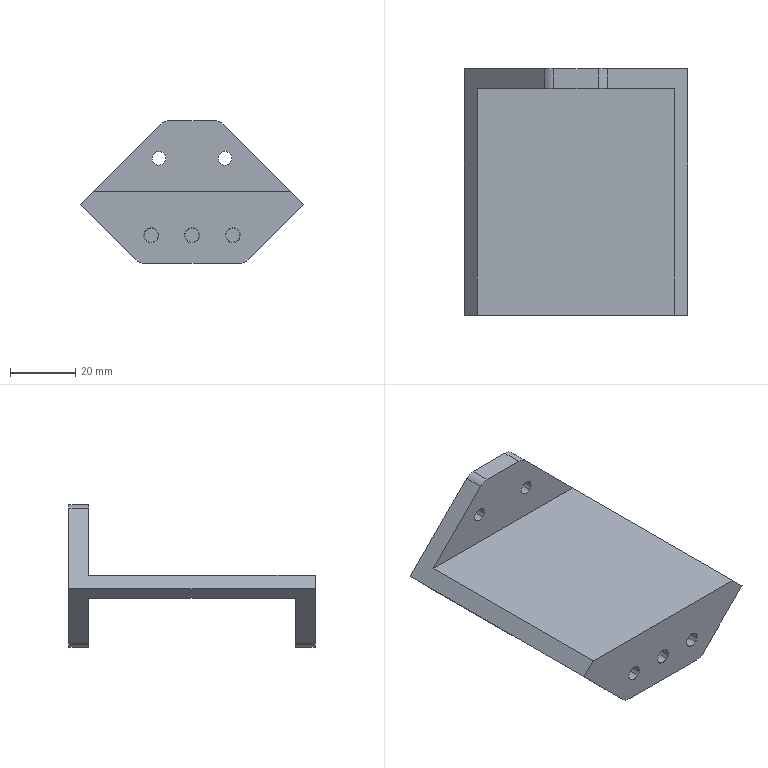NC program | NX | posted with a generic post | part box 68.307 x 75.3 x 43.668 mm
Lines 81 to 1013 of 6865:
(ADAPTIVE_MILLING_COPY_1 , TOOL : D10)
N160 T15 M6
N162 G54
N164 G17 G0 G90 X37.103 Y44.955 B0. C0. S9500 M3
N166 G43 Z30. H15
N168 Z-18.118
N170 G94 G1 Z-21.118 F1000.
N172 X35.037 Y43.518 F3000.
N174 G3 X34.603 Y42.688 R1.025
N176 G2 X37.336 Y37.585 R9.953
N178 X38.066 Y30.26 R36.076
N180 X38.139 Y16.26 R733.485
N182 G1 X38.14 Y-34.615
N184 X38.139 Y-34.74
N186 X38.135 Y-34.865
N188 X38.126 Y-34.99
N190 G2 X35.464 Y-39.18 R5.882
N192 X29.738 Y-41.187 R13.119
N194 X21.129 Y-41.612 R70.953
N196 G1 X19.879 Y-41.62
N198 X18.254 Y-41.627
N200 X16.004 Y-41.632
N202 X12.254 Y-41.636
N204 X0.629 Y-41.637
N206 X-31.121
N208 G2 X-35.385 Y-39.36 R5.577
N210 X-37.569 Y-33.972 R11.776
N212 X-38.106 Y-25.498 R55.2
N214 G1 X-38.116 Y-24.373
N216 X-38.125 Y-22.998
N218 X-38.132 Y-21.373
N220 X-38.136 Y-18.998
N222 X-38.139 Y-14.748
N224 X-38.14 Y7.252
N226 Y34.627
N228 X-38.135 Y34.877
N230 X-38.129 Y35.002
N232 X-38.118 Y35.126
N234 G2 X-36.378 Y38.941 R7.536
N236 G3 X-34.707 Y41.121 R26.03
N238 G1 X-34.661 Y41.238
N240 X-34.628 Y41.358
N242 X-34.606 Y41.481
N244 G3 X-35.484 Y42.483 R1.015
N246 G1 X-37.241 Y42.713
N248 G2 X-37.126 Y44.725 R1.01
N250 G1 Z-18.118
N252 G0 Z30.
N254 X37.103 Y45.944
N256 Z-18.118
N258 G1 Z-21.118 F1000.
N260 G2 X37.257 Y43.934 R1.01 F3000.
N262 G1 X35.476 Y43.689
N264 G3 X34.603 Y42.688 R1.015
N266 G2 X36.175 Y37.422 R55.918
N268 X37.056 Y27.727 R51.989
N270 X37.129 Y12.227 R790.085
N272 G1 Y-31.523
N274 X37.128 Y-31.648
N276 X37.126 Y-31.773
N278 X37.122 Y-31.898
N280 X37.116 Y-32.023
N282 X37.108 Y-32.147
N284 G2 X33.457 Y-37.968 R7.678
N286 X27.114 Y-40.112 R15.441
N288 X18.258 Y-40.59 R72.293
N290 G1 X17.133 Y-40.601
N292 X15.758 Y-40.61
N294 X14.008 Y-40.617
N296 X11.508 Y-40.622
N298 X7.508 Y-40.625
N300 X-4.742 Y-40.626
N302 X-27.992
N304 X-28.242 Y-40.624
N306 X-28.492 Y-40.615
N308 X-28.617 Y-40.606
N310 G2 X-34.521 Y-36.878 R7.68
N312 X-36.629 Y-30.521 R15.721
N314 X-37.101 Y-20.914 R80.427
N316 G1 X-37.11 Y-19.664
N318 X-37.117 Y-18.164
N320 X-37.123 Y-16.039
N322 X-37.127 Y-12.914
N324 X-37.129 Y-6.289
N326 Y31.711
N328 G2 X-35.536 Y37.429 R11.91
N330 G3 X-34.613 Y39.337 R10.413
N332 G1 X-34.603 Y39.41
N334 Y42.785
N336 G3 X-35.422 Y43.776 R1.017
N338 G1 X-36.981 Y44.078
N340 G3 X-37.127 Y42.077 R-1.01
N342 G1 Z-18.118
N344 G0 Z30.
N346 X37.103 Y45.449
N348 Z-18.118
N350 G1 Z-21.118 F1000.
N352 G2 X36.95 Y43.45 R-1.01 F3000.
N354 G1 X36.302 Y43.585
N356 X35.651 Y43.698
N358 G3 X34.603 Y42.688 R1.014
N360 X35.031 Y38.469 R20.052
N362 G2 X36.066 Y24.898 R85.494
N364 G1 X36.079 Y23.773
N366 X36.09 Y22.523
N368 X36.099 Y21.023
N370 X36.107 Y19.148
N372 X36.112 Y16.773
N374 X36.116 Y13.148
N376 X36.118 Y5.523
N378 X36.119 Y-28.852
N380 X36.117 Y-29.102
N382 X36.116 Y-29.227
N384 X36.113 Y-29.352
N386 X36.104 Y-29.602
N388 G2 X31.382 Y-37.073 R8.907
N390 X24.358 Y-39.151 R18.458
N392 X14.498 Y-39.586 R94.216
N394 G1 X13.123 Y-39.596
N396 X11.373 Y-39.604
N398 X9.123 Y-39.609
N400 X5.748 Y-39.613
N402 X-1.502 Y-39.615
N404 X-25.377
N406 G2 X-33.587 Y-34.86 R8.944
N408 X-35.64 Y-27.957 R18.351
N410 X-36.097 Y-16.972 R100.614
N412 G1 X-36.105 Y-15.347
N414 X-36.111 Y-13.222
N416 X-36.115 Y-10.222
N418 X-36.118 Y-4.597
N420 X-36.119 Y29.278
N422 X-36.116 Y29.528
N424 G2 X-34.835 Y35.861 R17.736
N426 X-34.752 Y38.412 R38.327
N428 G3 X-34.603 Y39.452 R4.992
N430 X-35.485 Y40.454 R1.015
N432 G1 X-37.225 Y40.677
N434 G2 X-37.127 Y42.689 R1.01
N436 G1 Z-18.118
N438 G0 Z30.
N440 X37.103 Y44.944
N442 Z-18.118
N444 G1 Z-21.118 F1000.
N446 G2 X37.27 Y42.934 R1.01 F3000.
N448 G1 X35.477 Y42.689
N450 G3 X34.603 Y41.688 R1.015
N452 G1 Y39.202
N454 X34.628 Y38.974
N456 G2 X34.815 Y37.63 R7.436
N458 G3 X35.002 Y27.258 R244.674
N460 G2 X35.107 Y4.883 R986.977
N462 G1 X35.108 Y-26.492
N464 X35.106 Y-26.867
N466 X35.102 Y-27.117
N468 X35.099 Y-27.242
N470 X35.09 Y-27.492
N472 X35.085 Y-27.616
N474 G2 X29.711 Y-36.054 R9.801
N476 X22.669 Y-38.093 R19.794
N478 X12.185 Y-38.573 R97.324
N480 G1 X10.81 Y-38.583
N482 X9.06 Y-38.591
N484 X6.685 Y-38.598
N486 X3.435 Y-38.602
N488 X-2.815 Y-38.604
N490 X-23.065 Y-38.605
N492 G2 X-29.137 Y-37.029 R10.422
N494 X-33.535 Y-30.968 R11.649
N496 X-34.886 Y-22.856 R30.289
N498 X-35.105 Y-7.234 R329.937
N500 G1 X-35.107 Y-1.359
N502 X-35.108 Y27.141
N504 X-35.107 Y27.391
N506 X-35.098 Y27.891
N508 X-35.089 Y28.266
N510 G2 X-34.789 Y31.456 R37.745
N512 G1 X-34.815 Y36.061
N514 G3 X-35.651 Y37.056 R1.016
N516 G1 X-37.096 Y37.309
N518 G3 X-37.25 Y35.304 R-1.01
N520 G1 Z-18.118
N522 G0 Z30.
N524 X37.314 Y36.803
N526 Z-18.118
N528 G1 Z-21.118 F1000.
N530 G2 X37.425 Y34.787 R1.01 F3000.
N532 G1 X35.735 Y34.636
N534 G3 X34.815 Y33.63 R1.015
N536 G2 X34.417 Y29.312 R15.253
N538 G3 X34.111 Y21.824 R59.692
N540 G1 X34.109 Y20.324
N542 X34.11 Y17.574
N544 X34.111 Y15.949
N546 X34.109 Y15.324
N548 X34.108 Y14.199
N550 X34.109 Y13.324
N552 X34.107 Y12.324
N554 X34.109 Y10.949
N556 X34.108 Y10.324
N558 Y8.949
N560 X34.11 Y7.949
N562 X34.108 Y7.074
N564 Y6.449
N566 X34.11 Y5.574
N568 X34.109 Y4.949
N570 Y3.574
N572 X34.111 Y2.574
N574 X34.109 Y1.824
N576 X34.11 Y0.824
N578 X34.111 Y0.199
N580 X34.108 Y-0.926
N582 X34.11 Y-2.051
N584 X34.108 Y-2.926
N586 X34.11 Y-4.176
N588 X34.107 Y-5.426
N590 X34.108 Y-6.176
N592 X34.107 Y-7.176
N594 X34.106 Y-7.676
N596 X34.108 Y-8.551
N598 X34.107 Y-9.551
N600 X34.109 Y-10.551
N602 X34.106 Y-11.676
N604 G2 X34.06 Y-26.05 R568.596
N606 X28.082 Y-35.076 R10.498
N608 X20.52 Y-37.113 R21.862
N610 X9.534 Y-37.564 R111.328
N612 G1 X8.034 Y-37.574
N614 X6.159 Y-37.582
N616 X3.659 Y-37.588
N618 X-0.091 Y-37.592
N620 X-7.841 Y-37.594
N622 X-20.966
N624 G2 X-26.461 Y-36.636 R12.841
N626 X-31.969 Y-30.748 R11.169
N628 X-33.698 Y-23.227 R24.56
N630 X-34.079 Y-10.987 R147.198
N632 G1 X-34.087 Y-8.987
N634 X-34.092 Y-6.487
N636 X-34.095 Y-2.362
N638 X-34.097 Y8.013
N640 Y25.263
N642 X-34.094 Y25.763
N644 X-33.996 Y28.759
N646 X-34.024 Y28.881
N648 X-34.065 Y28.999
N650 X-34.082 Y29.041
N652 X-34.133 Y29.128
N654 X-34.604 Y30.246
N656 X-34.64 Y30.379
N658 X-34.794 Y31.494
N660 G3 X-35.8 Y32.366 R1.015
N662 G1 X-36.601 Y32.355
N664 X-37.402 Y32.371
N666 G2 X-37.223 Y34.378 R1.01
N668 G1 Z-18.118
N670 G0 Z30.
N672 X37.315 Y33.119
N674 Z-18.118
N676 G1 Z-21.118 F1000.
N678 G2 X37.322 Y31.099 R1.01 F3000.
N680 G1 X35.564 Y31.057
N682 G3 X34.647 Y30.412 R1.02
N684 X33.318 Y24.736 R14.87
N686 X33.118 Y12.865 R216.262
N688 G1 X33.115 Y11.74
N690 X33.116 Y10.74
N692 X33.112 Y9.865
N694 X33.113 Y8.865
N696 Y8.49
N698 X33.111 Y7.615
N700 Y6.74
N702 X33.112 Y6.365
N704 X33.11 Y5.615
N706 X33.112 Y4.24
N708 X33.111 Y3.615
N710 X33.112 Y2.365
N712 X33.11 Y1.74
N714 Y1.365
N716 X33.111 Y0.24
N718 X33.109 Y-0.635
N720 X33.111 Y-1.885
N722 X33.108 Y-2.76
N724 X33.11 Y-3.76
N726 Y-4.135
N728 X33.108 Y-5.01
N730 X33.109 Y-5.76
N732 Y-6.26
N734 X33.107 Y-7.135
N736 X33.109 Y-8.135
N738 X33.106 Y-9.385
N740 X33.108 Y-10.135
N742 X33.107 Y-11.385
N744 X33.106 Y-12.01
N746 X33.108 Y-12.76
N748 Y-14.01
N750 X33.106 Y-14.76
N752 X33.108 Y-15.51
N754 X33.106 Y-16.76
N756 G2 X33.022 Y-24.758 R134.606
N758 X26.71 Y-34.011 R11.031
N760 X18.9 Y-36.089 R22.89
N762 X7.414 Y-36.553 R118.187
N764 G1 X5.914 Y-36.563
N766 X4.039 Y-36.57
N768 X1.539 Y-36.576
N770 X-2.086 Y-36.581
N772 X-9.086 Y-36.583
N774 X-19.086
N776 G2 X-24.733 Y-35.724 R14.855
N778 X-30.763 Y-29.68 R11.44
N780 X-32.652 Y-21.816 R24.499
N782 X-33.067 Y-9.077 R146.713
N784 G1 X-33.075 Y-7.077
N786 X-33.081 Y-4.452
N788 X-33.084 Y-0.452
N790 X-33.086 Y8.423
N792 Y23.673
N794 X-33.083 Y24.298
N796 G3 X-33.127 Y27.667 R21.347
N798 G1 X-33.167 Y27.785
N800 X-33.219 Y27.899
N802 X-33.281 Y28.007
N804 X-33.301 Y28.033
N806 X-33.319 Y28.051
N808 X-34.063 Y29.009
N810 X-34.126 Y29.116
N812 G3 X-35.154 Y29.604 R1.02
N814 G1 X-35.754 Y29.514
N816 X-36.351 Y29.402
N818 G3 X-36.005 Y27.435 R1.01
N820 G1 Z-18.118
N822 G0 Z30.
N824 X36.861 Y29.243
N826 Z-18.118
N828 G1 Z-21.118 F1000.
N830 G3 X36.183 Y31.023 R-1.01 F3000.
N832 G1 X34.34 Y29.451
N834 X34.197 Y29.253
N836 G3 X32.684 Y25.452 R7.841
N838 X32.174 Y17.225 R57.173
N840 G1 X32.162 Y16.225
N842 X32.149 Y14.85
N844 X32.14 Y13.475
N846 X32.132 Y11.6
N848 X32.125 Y8.725
N850 X32.122 Y5.85
N852 Y4.85
N854 X32.117 Y3.975
N856 X32.116 Y2.85
N858 X32.113 Y1.975
N860 Y1.35
N862 X32.114 Y0.6
N864 X32.111 Y-0.4
N866 X32.112 Y-1.525
N868 X32.11 Y-2.4
N870 X32.111 Y-3.4
N872 X32.11 Y-4.025
N874 X32.108 Y-4.775
N876 X32.11 Y-5.9
N878 X32.108 Y-6.9
N880 X32.109 Y-7.9
N882 X32.106 Y-9.15
N884 X32.108 Y-10.15
N886 X32.106 Y-11.525
N888 X32.108 Y-12.65
N890 X32.105 Y-14.025
N892 X32.108 Y-15.15
N894 X32.107 Y-15.9
N896 X32.108 Y-17.15
N898 X32.109 Y-17.525
N900 X32.107 Y-18.275
N902 X32.109 Y-19.525
N904 X32.106 Y-20.4
N906 G2 X31.543 Y-25.852 R19.752
N908 X25.441 Y-32.927 R11.455
N910 X17.639 Y-35.038 R23.236
N912 X6.405 Y-35.534 R110.524
N914 G1 X5.03 Y-35.545
N916 X3.405 Y-35.554
N918 X1.28 Y-35.561
N920 X-1.595 Y-35.567
N922 X-6.095 Y-35.571
N924 X-16.845 Y-35.572
N926 G2 X-22.54 Y-34.972 R19.104
N928 X-29.517 Y-28.751 R11.546
N930 X-31.546 Y-21.053 R23.59
N932 X-32.047 Y-8.694 R123.415
N934 G1 X-32.056 Y-7.194
N936 X-32.064 Y-5.194
N938 X-32.069 Y-2.569
N940 X-32.073 Y1.431
N942 X-32.075 Y9.681
N944 Y22.056
N946 G3 X-32.173 Y26.426 R33.371
N948 X-32.616 Y27.496 R1.749
N950 G1 X-33.22 Y27.953
N952 X-33.309 Y28.041
N954 G3 X-34.257 Y28.304 R1.024
N956 G1 X-34.789 Y28.179
N958 X-35.315 Y28.033
N960 G3 X-34.888 Y26.097 R1.01
N962 G1 Z-18.118
N964 G0 Z30.
N966 X36.224 Y27.789
N968 Z-18.118
N970 G1 Z-21.118 F1000.
N972 G3 X35.767 Y29.712 R-1.01 F3000.
N974 G1 X34.136 Y28.939
N976 X33.929 Y28.804
N978 X33.757 Y28.627
N980 G3 X32.666 Y27.098 R11.091
N982 X31.503 Y22.133 R14.995
N984 X31.154 Y11.642 R125.927
N986 G1 X31.145 Y9.892
N988 X31.138 Y7.642
N990 X31.132 Y6.892
N992 X31.128 Y5.892
N994 X31.127 Y5.142
N996 X31.123 Y4.517
N998 X31.121 Y3.392
N1000 Y2.767
N1002 X31.117 Y2.017
N1004 X31.116 Y0.767
N1006 X31.113 Y-0.108
N1008 X31.114 Y-1.233
N1010 X31.112 Y-1.983
N1012 Y-3.108
N1014 Y-3.733
N1016 X31.11 Y-4.608
N1018 X31.111 Y-5.608
N1020 X31.109 Y-6.483
N1022 Y-7.358
N1024 X31.11 Y-7.733
N1026 X31.107 Y-8.858
N1028 X31.108 Y-9.858
N1030 G2 X31.038 Y-21.232 R335.421
N1032 X28.284 Y-28.715 R12.219
N1034 X21.359 Y-32.99 R14.44
N1036 X12.48 Y-34.319 R37.619
N1038 X-3.391 Y-34.556 R349.331
N1040 X-17.641 Y-34.513 R594.266
N1042 X-24.955 Y-31.983 R12.297
N1044 X-29.426 Y-25.047 R14.176
N1046 X-30.802 Y-16.301 R36.508
N1048 X-31.061 Y1.32 R359.385
N1050 G1 X-31.064 Y6.82
N1052 X-31.065 Y22.32
N1054 X-31.068 Y22.945
N1056 X-31.075 Y23.319
N1058 X-31.084 Y23.694
N1060 G3 X-31.548 Y26.64 R8.286
N1062 X-32.253 Y27.221 R1.49
N1064 G1 X-32.652 Y27.523
N1066 G3 X-33.174 Y27.724 R1.066
N1068 G1 X-33.903 Y27.794
N1070 X-34.633 Y27.836
N1072 G3 X-34.539 Y25.82 R1.01
N1074 G1 Z-18.118
N1076 G0 Z30.
N1078 X35.268 Y26.489
N1080 Z-18.118
N1082 G1 Z-21.118 F1000.
N1084 G3 X35.063 Y28.49 R-1.01 F3000.
N1086 G1 X34.312 Y28.348
N1088 X33.566 Y28.183
N1090 X33.424 Y28.113
N1092 X33.29 Y28.029
N1094 G3 X31.427 Y25.289 R5.112
N1096 X30.391 Y18.891 R25.27
N1098 X30.128 Y4.145 R316.596
N1100 G1 X30.118 Y2.395
N1102 Y1.52
N1104 X30.115 Y-0.105
N1106 X30.113 Y-0.73
N1108 X30.114 Y-1.48
N1110 X30.112 Y-2.48
N1112 X30.113 Y-3.48
N1114 X30.111 Y-4.23
N1116 Y-5.105
N1118 Y-5.48
N1120 X30.109 Y-6.355
N1122 X30.11 Y-7.605
N1124 X30.107 Y-8.855
N1126 X30.108 Y-9.73
N1128 X30.107 Y-10.605
N1130 X30.106 Y-11.105
N1132 X30.109 Y-12.23
N1134 G2 X29.987 Y-20.352 R125.54
N1136 X22.838 Y-30.872 R12.218
N1138 X14.779 Y-32.993 R24.668
N1140 X2.171 Y-33.518 R124.82
N1142 X-15.954 Y-33.511 R865.658
N1144 X-22.742 Y-31.641 R13.493
N1146 X-27.966 Y-24.968 R13.34
N1148 X-29.659 Y-16.667 R30.391
N1150 X-30.034 Y-3.426 R186.103
N1152 G1 X-30.042 Y-1.301
N1154 X-30.048 Y1.574
N1156 X-30.052 Y5.949
N1158 X-30.054 Y15.074
N1160 Y19.324
N1162 X-30.059 Y20.199
N1164 G3 X-30.381 Y25.18 R25.808
N1166 X-31.141 Y26.718 R2.586
N1168 G1 X-31.246 Y26.786
N1170 X-31.276 Y26.803
N1172 X-32.087 Y27.133
N1174 G3 X-32.759 Y27.165 R1.049
N1176 G1 X-33.258 Y27.018
N1178 X-33.751 Y26.851
N1180 G3 X-33.284 Y24.937 R1.011
N1182 G1 Z-18.118
N1184 G0 Z30.
N1186 X34.788 Y26.047
N1188 Z-18.118
N1190 G1 Z-21.118 F1000.
N1192 G3 X34.666 Y28.062 R-1.01 F3000.
N1194 G1 X33.275 Y27.906
N1196 X33.078 Y27.83
N1198 X32.897 Y27.72
N1200 G3 X30.538 Y24.448 R5.822
N1202 X29.415 Y17.559 R27.189
N1204 X29.132 Y2.439 R319.398
N1206 G1 X29.123 Y0.189
N1208 X29.118 Y-2.061
N1210 X29.117 Y-4.311
N1212 Y-5.436
N1214 X29.113 Y-6.186
N1216 X29.112 Y-7.311
N1218 Y-7.811
N1220 X29.109 Y-8.811
N1222 X29.111 Y-10.061
N1224 X29.108 Y-11.061
N1226 X29.11 Y-12.186
N1228 X29.107 Y-13.186
N1230 X29.094 Y-15.936
N1232 G2 X28.418 Y-22.128 R22.321
N1234 X21.816 Y-29.738 R12.42
N1236 X13.652 Y-31.947 R24.751
N1238 X1.42 Y-32.499 R117.274
N1240 X-14.704 Y-32.489 R561.42
N1242 X-21.815 Y-30.425 R13.689
N1244 X-26.907 Y-23.79 R13.679
N1246 X-28.642 Y-15.245 R30.728
N1248 X-29.026 Y-1.254 R194.787
N1250 G1 X-29.033 Y0.996
N1252 X-29.038 Y4.121
N1254 X-29.042 Y8.996
N1256 X-29.043 Y16.371
N1258 X-29.05 Y17.496
N1260 X-29.067 Y19.621
N1262 G3 X-29.526 Y24.838 R22.415
N1264 X-30.382 Y26.471 R2.961
N1266 X-31.357 Y26.836 R10.192
N1268 X-31.873 Y26.902 R1.123
N1270 G1 X-32.515 Y26.82
N1272 X-33.153 Y26.714
N1274 G3 X-32.831 Y24.741 R1.01
N1276 G1 Z-18.118
N1278 G0 Z30.
N1280 X34.981 Y26.206
N1282 Z-18.118
N1284 G1 Z-21.118 F1000.
N1286 G3 X34.595 Y28.158 R-1.01 F3000.
N1288 G1 X32.46 Y27.333
N1290 X32.311 Y27.261
N1292 G3 X30.306 Y25.268 R4.021
N1294 X28.746 Y19.636 R16.673
N1296 X28.204 Y8.78 R99.972
N1298 X28.113 Y-9.594 R973.755
N1300 G2 X27.955 Y-17.841 R113.139
N1302 X23.743 Y-26.625 R12.747
N1304 X16.159 Y-30.269 R17.281
N1306 X5.985 Y-31.372 R53.604
N1308 X-13.263 Y-31.478 R476.02
N1310 X-20.311 Y-29.596 R14.516
N1312 X-25.873 Y-22.573 R13.807
N1314 X-27.623 Y-13.903 R31.281
N1316 X-28.017 Y1.088 R206.595
N1318 G1 X-28.024 Y3.588
N1320 X-28.029 Y7.088
N1322 X-28.032 Y13.088
N1324 Y13.463
N1326 X-28.052 Y16.213
N1328 X-28.068 Y18.338
N1330 G3 X-28.567 Y24.179 R26.79
N1332 X-29.686 Y26.371 R4.218
N1334 X-30.865 Y26.658 R2.546
N1336 X-31.459 Y26.552 R1.057
N1338 G1 X-31.875 Y26.337
N1340 X-32.282 Y26.106
N1342 G3 X-31.659 Y24.291 R1.011
N1344 G1 Z-18.118
N1346 G0 Z30.
N1348 X33.611 Y25.126
N1350 Z-18.118
N1352 G1 Z-21.118 F1000.
N1354 G3 X33.619 Y27.146 R1.01 F3000.
N1356 G1 X32.231 Y27.165
N1358 X31.959 Y27.093
N1360 G3 X29.585 Y24.991 R4.235
N1362 X27.862 Y19.28 R16.365
N1364 X27.241 Y9.18 R84.951
N1366 X27.108 Y-10.569 R964.82
N1368 G2 X26.848 Y-17.435 R57.946
N1370 X19.401 Y-27.688 R12.872
N1372 X11.355 Y-29.874 R25.642
N1374 X-0.374 Y-30.464 R109.467
N1376 X-12.248 Y-30.448 R275.556
N1378 X-19.164 Y-28.545 R14.509
N1380 X-24.773 Y-21.555 R13.933
N1382 X-26.594 Y-12.773 R31.649
N1384 X-27.001 Y1.342 R191.743
N1386 G3 X-27.13 Y19.591 R855.724
N1388 X-27.975 Y24.75 R16.699
N1390 X-29.092 Y26.369 R3.211
N1392 X-30.132 Y26.566 R3.528
N1394 X-30.926 Y26.322 R1.035
N1396 G1 X-31.528 Y25.773
N1398 G3 X-30.732 Y24.124 R1.011
N1400 G1 Z-18.118
N1402 G0 Z30.
N1404 X33.407 Y25.02
N1406 Z-18.118
N1408 G1 Z-21.118 F1000.
N1410 G3 X33.325 Y27.037 R-1.01 F3000.
N1412 G1 X31.706 Y26.927
N1414 X31.542 Y26.898
N1416 X31.383 Y26.851
N1418 G3 X28.849 Y24.74 R4.317
N1420 X26.996 Y19.07 R16.087
N1422 X26.279 Y9.229 R74.179
N1424 X26.098 Y-11.02 R981.844
N1426 G2 X25.59 Y-17.613 R32.102
N1428 X18.427 Y-26.564 R12.995
N1430 X9.781 Y-28.893 R25.797
N1432 X-3.075 Y-29.466 R126.906
N1434 X-11.697 Y-29.38 R118.284
N1436 X-19.714 Y-26.281 R13.434
N1438 X-24.25 Y-18.934 R15.613
N1440 X-25.722 Y-9.446 R40.118
N1442 X-26.004 Y7.55 R338.738
N1444 G3 X-26.178 Y19.422 R302.178
N1446 X-27.176 Y24.678 R16.433
N1448 X-28.416 Y26.366 R3.718
N1450 X-29.57 Y26.5 R2.457
N1452 X-30.257 Y26.23 R1.039
N1454 G1 X-30.559 Y25.952
N1456 X-30.848 Y25.661
N1458 G3 X-30.041 Y24.039 R1.012
N1460 G1 Z-18.118
N1462 G0 Z30.
N1464 X31.717 Y24.301
N1466 Z-18.118
N1468 G1 Z-21.118 F1000.
N1470 G3 X32.187 Y26.203 R1.011 F3000.
N1472 G1 X31.369 Y26.624
N1474 X31.141 Y26.671
N1476 X30.907
N1478 G3 X28.713 Y25.364 R3.249
N1480 X26.485 Y20.523 R12.039
N1482 X25.41 Y11.602 R46.532
N1484 X25.113 Y-8.77 R619.479
N1486 G2 X24.713 Y-15.75 R44.682
N1488 X17.198 Y-25.578 R13.228
N1490 X9.163 Y-27.8 R25.491
N1492 X-3.564 Y-28.444 R112.612
N1494 X-11.307 Y-28.276 R67.098
N1496 X-22.16 Y-20.492 R13.227
N1498 X-24.388 Y-11.944 R26.869
N1500 X-24.948 Y0.163 R121.758
N1502 G3 X-25.146 Y17.911 R801.399
N1504 X-26.057 Y23.822 R22.03
N1506 X-27.626 Y26.329 R5.19
N1508 X-28.879 Y26.5 R2.315
N1510 X-29.731 Y26.032 R1.024
N1512 G1 X-30.114 Y25.405
N1514 G3 X-29.18 Y24. R1.012
N1516 G1 Z-18.118
N1518 G0 Z30.
N1520 X31.405 Y24.234
N1522 Z-18.118
N1524 G1 Z-21.118 F1000.
N1526 G3 X31.947 Y26.094 R1.011 F3000.
N1528 G1 X31.213 Y26.554
N1530 G3 X30.659 Y26.638 R1.066
N1532 X27.985 Y25.216 R3.62
N1534 X25.631 Y20.296 R12.311
N1536 X24.454 Y11.264 R45.018
N1538 X24.13 Y-6.607 R501.202
N1540 G2 X23.818 Y-13.845 R62.82
N1542 X15.9 Y-24.632 R13.495
N1544 X7.226 Y-26.872 R27.273
N1546 X-8.754 Y-27.37 R126.187
N1548 X-16.215 Y-25.158 R14.819
N1550 X-21.786 Y-17.816 R14.727
N1552 X-23.565 Y-8.769 R34.191
N1554 X-23.966 Y4.472 R196.489
N1556 G3 X-24.193 Y17.844 R346.993
N1558 X-25.303 Y23.97 R20.609
N1560 X-26.882 Y26.329 R5.314
N1562 X-28.134 Y26.5 R2.318
N1564 X-29.093 Y25.806 R1.017
N1566 G1 X-29.291 Y25.157
N1568 G3 X-28.288 Y24. R1.014
N1570 G1 Z-18.118
N1572 G0 Z30.
N1574 X31.187 Y24.203
N1576 Z-18.118
N1578 G1 Z-21.118 F1000.
N1580 G3 X31.508 Y26.169 R1.01 F3000.
N1582 G1 X30.929 Y26.368
N1584 X30.346 Y26.55
N1586 X30.039 Y26.557
N1588 G3 X27.265 Y25.113 R3.784
N1590 X24.852 Y20.359 R12.313
N1592 X23.539 Y11.599 R40.98
N1594 X23.13 Y-6.394 R407.732
N1596 G2 X22.704 Y-13.373 R44.165
N1598 X14.884 Y-23.557 R13.593
N1600 X6.096 Y-25.85 R27.468
N1602 X-8.008 Y-26.307 R95.775
N1604 X-16.112 Y-23.398 R14.202
N1606 X-21.004 Y-15.992 R15.623
N1608 X-22.617 Y-6.656 R37.799
N1610 X-22.998 Y8.587 R301.033
N1612 G3 X-23.326 Y18.704 R127.219
N1614 X-24.729 Y24.506 R17.35
N1616 X-26.165 Y26.363 R4.667
N1618 X-27.493 Y26.5 R2.906
N1620 X-28.393 Y25.936 R1.011
N1622 X-28.393 Y25.022 Z-21.071 R1.149
N1624 G1 X-28.082 Y24.01 Z-21.018
N1626 X-27.508 Y22.117
N1628 X-25.544 Y-9.189
N1630 G3 X-24.219 Y-16.025 R28.277
N1632 X-22.432 Y-20.546 R35.526
N1634 X-20.003 Y-24.143 R15.899
N1636 X-15.516 Y-27.42 R14.813
N1638 X-10.183 Y-29.01 R15.281
N1640 X-4.588 Y-29.55 R112.514
N1642 X-0.848 Y-29.517 R26.184
N1644 G1 X3.076 Y-29.199
N1646 X6.997 Y-28.854
N1648 G3 X12.98 Y-27.638 R34.154
N1650 X18.335 Y-25.027 R22.395
N1652 X23.493 Y-20.106 R17.239
N1654 X25.246 Y-16.169 R13.47
N1656 X25.763 Y-13.458 R17.705
N1658 G1 X29.583 Y22.093
N1660 X30.167 Y24.028
N1662 X30.372 Y24.691 Z-21.053
N1664 X30.559 Y25.359 Z-21.087
N1666 G3 X30.46 Y25.953 Z-21.118 R1.046
N1668 X29.569 Y26.5 R1.011
N1670 X26.883 Y25.389 R3.446
N1672 X24.194 Y20.795 R11.281
N1674 X22.637 Y11.954 R36.434
N1676 X22.177 Y-3.162 R265.529
N1678 G2 X21.86 Y-11.152 R82.32
N1680 X17.695 Y-19.874 R13.894
N1682 X9.906 Y-23.932 R17.754
N1684 X-0.243 Y-25.23 R49.929
N1686 X-7.984 Y-25.157 R50.512
N1688 X-18.918 Y-17.437 R13.526
N1690 X-21.299 Y-8.675 R26.723
N1692 X-21.923 Y4.054 R126.921
N1694 G3 X-22.247 Y17.049 R279.838
N1696 X-23.525 Y23.651 R23.084
N1698 X-25.307 Y26.322 R6.139
N1700 X-25.821 Y26.5 R3.376
N1702 G1 X-26.696
N1704 G3 X-27.596 Y25.936 R1.011
N1706 X-27.595 Y25.022 Z-21.071 R1.149
N1708 G1 X-27.284 Y24.011 Z-21.018
N1710 X-26.71 Y22.117
N1712 X-25.175 Y-2.328
N1714 G3 X-24.089 Y-10.993 R71.2
N1716 G1 X-23.497 Y-14.059
N1718 G3 X-21.205 Y-19.691 R19.518
N1720 X-18.094 Y-23.732 R21.708
N1722 X-15.001 Y-25.989 R13.44
N1724 X-7.449 Y-28.4 R21.823
N1726 X-4.963 Y-28.511 R18.106
N1728 G1 X-1.32 Y-28.413
N1730 X2.322 Y-28.292
N1732 G3 X10.51 Y-26.934 R39.564
N1734 X14.614 Y-25.464 R42.308
N1736 X16.981 Y-24.181 R17.205
N1738 X19.155 Y-22.649 R22.033
N1740 X21.85 Y-19.73 R17.352
N1742 X23.795 Y-15.858 R15.975
N1744 X24.9 Y-11.007 R24.699
N1746 G1 X29.069 Y22.
N1748 X29.104 Y22.164
N1750 X29.653 Y23.979
N1752 X30.057 Y25.349 Z-21.089
N1754 G3 X29.982 Y25.907 Z-21.118 R1.054
N1756 X29.069 Y26.5 R1.01
N1758 X26.145 Y25.336 R3.714
N1760 X23.306 Y20.543 R11.777
N1762 X21.704 Y11.836 R36.423
N1764 X21.189 Y-2.902 R236.744
N1766 G2 X20.809 Y-10.388 R67.198
N1768 X12.703 Y-21.489 R13.917
N1770 X3.919 Y-23.8 R27.715
N1772 X-6.435 Y-24.146 R55.099
N1774 X-17.925 Y-16.26 R13.645
N1776 X-20.271 Y-7.614 R27.225
N1778 X-20.917 Y4.989 R125.921
N1780 G3 X-21.292 Y16.856 R211.787
N1782 X-22.7 Y23.685 R22.978
N1784 X-24.517 Y26.333 R6.168
N1786 X-25.014 Y26.5 R4.9
N1788 G1 X-25.889
N1790 G3 X-26.789 Y25.936 R1.011
N1792 X-26.788 Y25.023 Z-21.071 R1.149
N1794 G1 X-26.478 Y24.011 Z-21.018
N1796 X-25.903 Y22.115
N1798 X-24.475 Y0.797
N1800 G3 X-23.164 Y-9.095 R77.526
N1802 G1 X-22.395 Y-12.891
N1804 G3 X-20.512 Y-18.027 R21.219
N1806 G1 X-19.749 Y-19.333
N1808 X-18.934 Y-20.609
N1810 G3 X-15.828 Y-23.743 R13.185
N1812 X-12.061 Y-25.928 R21.419
N1814 X-8.462 Y-26.872 R11.91
N1816 X-1.616 Y-27.434 R169.237
N1818 X2.111 Y-27.261 R19.335
N1820 G1 X6.188 Y-26.648
N1822 G3 X12.086 Y-25.061 R35.891
N1824 X17.267 Y-22.358 R27.893
N1826 X19.235 Y-20.639 R13.827
N1828 X21.424 Y-17.65 R12.134
N1830 G1 X21.995 Y-16.546
N1832 X22.521 Y-15.419
N1834 G3 X23.491 Y-12.147 R17.874
N1836 G1 X23.755 Y-10.769
N1838 X23.98 Y-9.385
N1840 X28.444 Y22.
N1842 X28.724 Y22.992
N1844 X29.028 Y23.977
N1846 X29.432 Y25.35 Z-21.09
N1848 G3 X29.358 Y25.906 Z-21.118 R1.054
N1850 X28.444 Y26.5 R1.01
N1852 X25.401 Y25.304 R3.881
N1854 X22.414 Y20.311 R12.249
N1856 X20.76 Y11.614 R36.933
N1858 X20.205 Y-2.373 R224.037
N1860 G2 X19.719 Y-9.85 R52.617
N1862 X11.657 Y-20.446 R14.03
N1864 X3.249 Y-22.726 R27.314
N1866 X-5.852 Y-23.014 R40.642
N1868 X-16.754 Y-15.437 R13.552
N1870 X-19.156 Y-7.195 R25.852
N1872 X-19.88 Y4.401 R104.762
N1874 G3 X-20.296 Y16.267 R233.658
N1876 X-21.715 Y23.351 R25.363
N1878 X-23.598 Y26.259 R7.111
N1880 X-24.2 Y26.5 R1.72
N1882 G1 X-25.075
N1884 G3 X-25.975 Y25.936 R1.011
N1886 X-25.975 Y25.023 Z-21.071 R1.149
N1888 G1 X-25.664 Y24.011 Z-21.018
N1890 X-25.089 Y22.112
N1892 X-23.65 Y2.051
N1894 G3 X-22.249 Y-7.826 R72.571
N1896 G1 X-21.541 Y-11.081
N1898 G3 X-19.498 Y-16.738 R29.114
N1900 X-17.837 Y-19.355 R17.71
N1902 X-15.938 Y-21.67 R26.322
N1904 X-12.867 Y-23.992 R13.414
N1906 X-9.994 Y-25.165 R11.553
N1908 G1 X-6.766 Y-25.972
N1910 G3 X-4.144 Y-26.416 R19.87
N1912 G1 X-3.398 Y-26.443
N1914 X-2.652 Y-26.427
N1916 G3 X2.325 Y-26.013 R69.097
N1918 X7.24 Y-25.133 R69.097
N1920 X13.687 Y-22.875 R25.582
N1922 X16.248 Y-21.134 R16.059
N1924 X18.498 Y-19.158 R27.895
N1926 X19.746 Y-17.61 R11.158
N1928 G1 X20.367 Y-16.674
N1930 X20.952 Y-15.716
N1932 G3 X22.276 Y-11.976 R12.016
N1934 X25.169 Y5.277 R988.549
N1936 G1 X27.819 Y22.
N1938 X28.405 Y23.98
N1940 X28.807 Y25.351 Z-21.089
N1942 G3 X28.731 Y25.909 Z-21.118 R1.054
N1944 X27.819 Y26.5 R1.01
N1946 X24.654 Y25.284 R4.021
N1948 X21.601 Y20.329 R12.394
N1950 X19.795 Y11.156 R36.85
N1952 X19.246 Y-1.204 R197.914
N1954 G2 X18.755 Y-8.557 R57.864
N1956 X10.408 Y-19.506 R14.201
N1958 X1.484 Y-21.781 R28.655
N1960 X-6.236 Y-21.69 R26.051
N1962 X-15.635 Y-14.51 R13.427
N1964 X-18.156 Y-5.918 R25.837
N1966 X-18.865 Y4.928 R105.461
N1968 G3 X-19.388 Y16.664 R176.323
N1970 X-21.004 Y23.702 R23.865
N1972 X-22.863 Y26.327 R6.519
N1974 X-23.369 Y26.5 R3.843
N1976 G1 X-24.244
N1978 G3 X-25.144 Y25.936 R1.011
N1980 X-25.144 Y25.023 Z-21.071 R1.149
N1982 G1 X-24.834 Y24.011 Z-21.018
N1984 X-24.259 Y22.109
N1986 X-23.325 Y10.166
N1988 G3 X-21.663 Y-3.47 R159.149
N1990 G1 X-21.224 Y-6.121
N1992 X-20.766 Y-8.768
N1994 G3 X-19.291 Y-13.971 R31.77
N1996 X-17.048 Y-18.197 R20.736
N1998 X-14.549 Y-20.937 R15.593
N2000 G1 X-13.217 Y-22.067
N2002 G3 X-10.395 Y-23.628 R11.317
N2004 X-6.185 Y-24.732 R20.144
N2006 G1 X-4.946 Y-24.853
N2008 X-1.566 Y-25.043
N2010 G3 X4.36 Y-24.549 R27.993
N2012 X10.93 Y-22.626 R31.512
N2014 X14.378 Y-20.649 R19.748
N2016 X17.075 Y-18.447 R21.762
N2018 X20.901 Y-12.134 R15.85